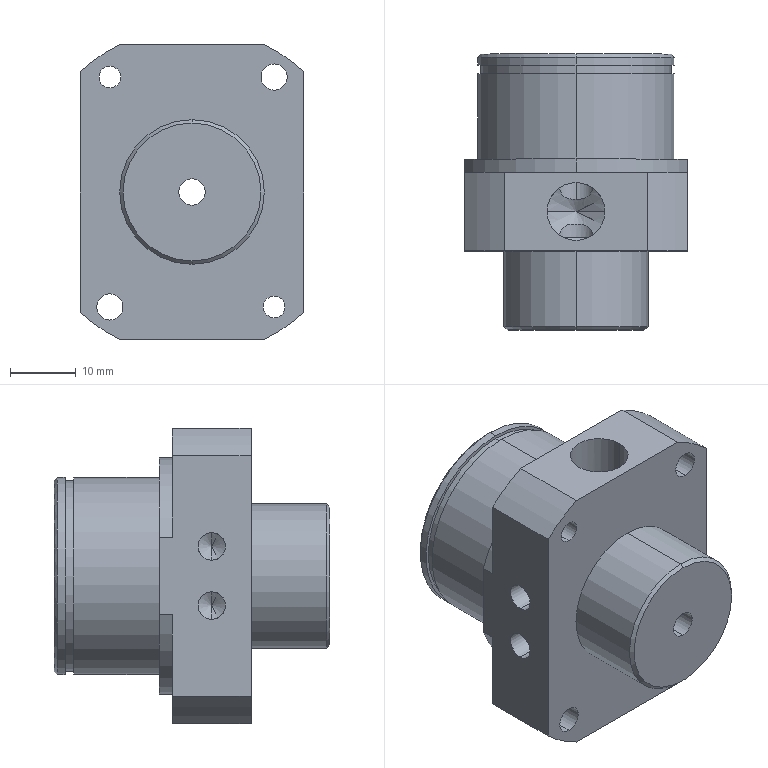Part | SolidWorks | features ICE 10, HoleWzd 7, Chamfer 2, Revolution 1 | 1 solid | 120 faces | box 34 x 42 x 45 mm | volume 29276 mm3 | cylinder 72 | cone 30 | plane 18 | commonest cylinder face diameters 4 x22 4.2 x16 6 x7 3.3 x4 6.8 x4 8.8 x4